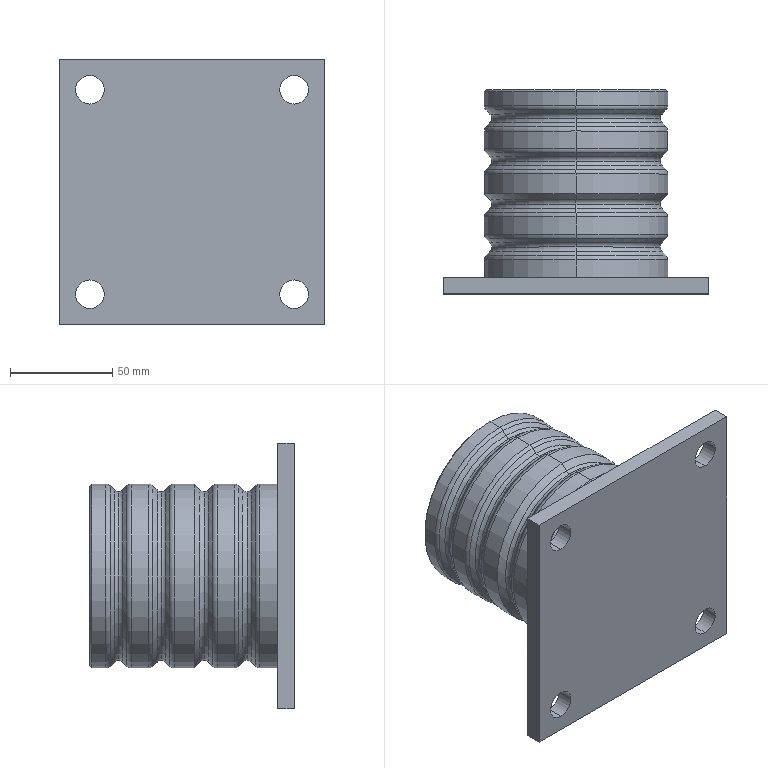Part | SolidWorks | features Chamfer 1, Extrusion 1, Fillet 1, ICE 1, RevCut 1 | 1 solid | 73 faces | box 130 x 100 x 130 mm | volume 689791 mm3 | torus 30 | cylinder 18 | cone 18 | plane 7 | commonest cylinder face diameters 90 x10 14 x8